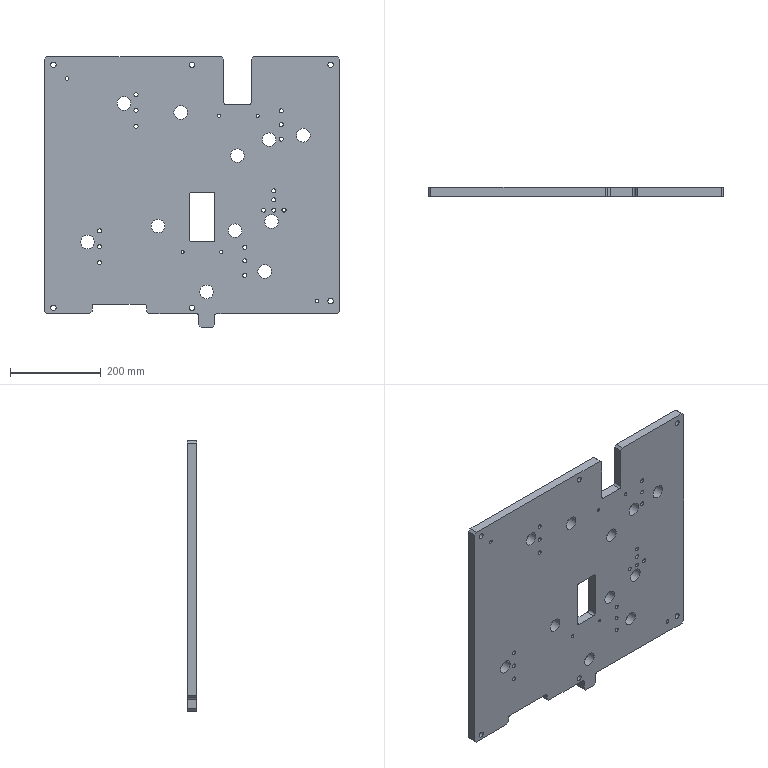Part | NX | features BREP 1 | 1 solid | 230 faces | box 650 x 20 x 595 mm | volume 6841559 mm3 | cylinder 124 | cone 68 | plane 38 | commonest cylinder face diameters 6 x52 9 x17 5 x16 30 x11 10 x10 12 x6